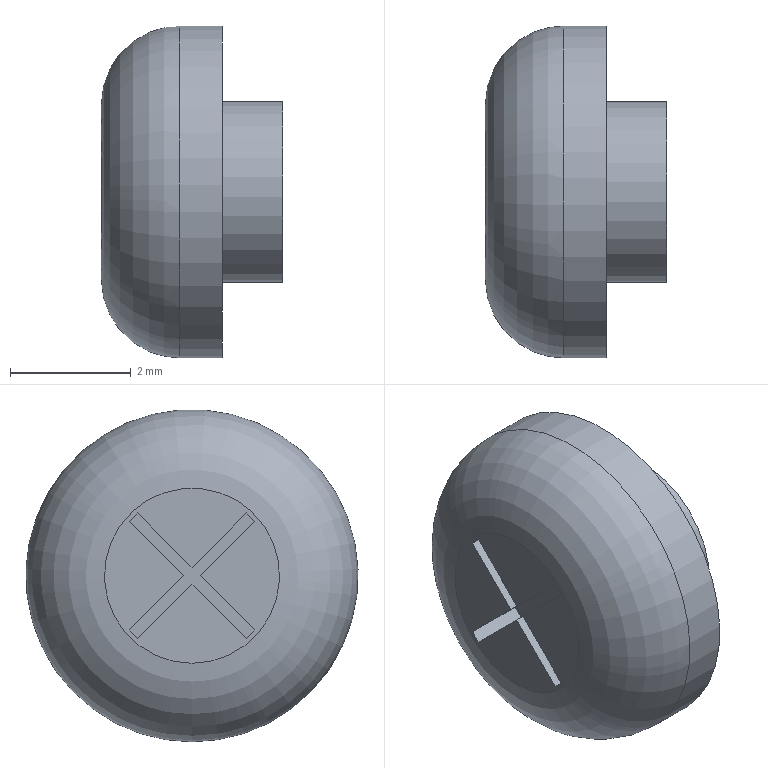Part | STEP file | 1 solid | 19 faces | box 3 x 5.5 x 5.5 mm | volume 47.924 mm3 | plane 16 | cylinder 2 | torus 1 | commonest cylinder face diameters 3 x1 5.5 x1
STEP:
#1=CARTESIAN_POINT('',(0.,0.,0.));
#2=DIRECTION('',(0.,0.,1.));
#3=DIRECTION('',(1.,0.,0.));
#4=AXIS2_PLACEMENT_3D('',#1,#2,#3);
#5=CARTESIAN_POINT('',(0.,0.,-1.5));
#6=VERTEX_POINT('',#5);
#7=CARTESIAN_POINT('',(0.,0.,0.));
#8=DIRECTION('',(-1.,0.,0.));
#9=DIRECTION('',(0.,0.,-1.));
#10=AXIS2_PLACEMENT_3D('',#7,#8,#9);
#11=CIRCLE('',#10,1.5);
#12=CARTESIAN_POINT('',(0.,0.,0.));
#13=DIRECTION('',(1.,0.,0.));
#14=DIRECTION('',(0.,0.,-1.));
#15=AXIS2_PLACEMENT_3D('',#12,#13,#14);
#16=PLANE('',#15);
#17=CARTESIAN_POINT('',(1.5,0.));
#18=CARTESIAN_POINT('',(1.5,-2.598));
#19=CARTESIAN_POINT('',(-0.75,-1.299));
#20=CARTESIAN_POINT('',(-3.,0.));
#21=CARTESIAN_POINT('',(-0.75,1.299));
#22=CARTESIAN_POINT('',(1.5,2.598));
#23=CARTESIAN_POINT('',(1.5,0.));
#24=(BOUNDED_CURVE()B_SPLINE_CURVE(2,(#17,#18,#19,#20,#21,#22,#23),.UNSPECIFIED.,.T.,.F.)B_SPLINE_CURVE_WITH_KNOTS((1,2,2,2,2,1),(-2.094,0.,2.094,4.189,6.283,8.378),.UNSPECIFIED.)CURVE()GEOMETRIC_REPRESENTATION_ITEM()RATIONAL_B_SPLINE_CURVE((1.,0.5,1.,0.5,1.,0.5,1.))REPRESENTATION_ITEM(''));
#25=(GEOMETRIC_REPRESENTATION_CONTEXT(2)PARAMETRIC_REPRESENTATION_CONTEXT()REPRESENTATION_CONTEXT('',''));
#26=DEFINITIONAL_REPRESENTATION('',(#24),#25);
#27=PCURVE('',#16,#26);
#28=CARTESIAN_POINT('',(-2.15,0.,0.));
#29=DIRECTION('',(1.,0.,0.));
#30=DIRECTION('',(0.,0.,-1.));
#31=AXIS2_PLACEMENT_3D('',#28,#29,#30);
#32=CYLINDRICAL_SURFACE('',#31,1.5);
#33=CARTESIAN_POINT('',(6.283,2.15));
#34=DIRECTION('',(-1.,0.));
#35=VECTOR('',#34,1.);
#36=LINE('',#33,#35);
#37=(GEOMETRIC_REPRESENTATION_CONTEXT(2)PARAMETRIC_REPRESENTATION_CONTEXT()REPRESENTATION_CONTEXT('',''));
#38=DEFINITIONAL_REPRESENTATION('',(#36),#37);
#39=PCURVE('',#32,#38);
#40=SURFACE_CURVE('',#11,(#27,#39),.PCURVE_S1.);
#41=EDGE_CURVE('',#6,#6,#40,.T.);
#42=ORIENTED_EDGE('',*,*,#41,.T.);
#43=EDGE_LOOP('',(#42));
#44=FACE_BOUND('',#43,.T.);
#45=CARTESIAN_POINT('',(0.,0.,-2.75));
#46=VERTEX_POINT('',#45);
#47=CARTESIAN_POINT('',(0.,0.,0.));
#48=DIRECTION('',(1.,0.,0.));
#49=DIRECTION('',(0.,0.,-1.));
#50=AXIS2_PLACEMENT_3D('',#47,#48,#49);
#51=CIRCLE('',#50,2.75);
#52=CARTESIAN_POINT('',(0.,0.));
#53=DIRECTION('',(1.,0.));
#54=AXIS2_PLACEMENT_2D('',#52,#53);
#55=CIRCLE('',#54,2.75);
#56=(GEOMETRIC_REPRESENTATION_CONTEXT(2)PARAMETRIC_REPRESENTATION_CONTEXT()REPRESENTATION_CONTEXT('',''));
#57=DEFINITIONAL_REPRESENTATION('',(#55),#56);
#58=PCURVE('',#16,#57);
#59=CARTESIAN_POINT('',(-2.15,0.,0.));
#60=DIRECTION('',(1.,0.,0.));
#61=DIRECTION('',(0.,0.,-1.));
#62=AXIS2_PLACEMENT_3D('',#59,#60,#61);
#63=CYLINDRICAL_SURFACE('',#62,2.75);
#64=CARTESIAN_POINT('',(0.,2.15));
#65=DIRECTION('',(1.,0.));
#66=VECTOR('',#65,1.);
#67=LINE('',#64,#66);
#68=(GEOMETRIC_REPRESENTATION_CONTEXT(2)PARAMETRIC_REPRESENTATION_CONTEXT()REPRESENTATION_CONTEXT('',''));
#69=DEFINITIONAL_REPRESENTATION('',(#67),#68);
#70=PCURVE('',#63,#69);
#71=SURFACE_CURVE('',#51,(#58,#70),.PCURVE_S1.);
#72=EDGE_CURVE('',#46,#46,#71,.T.);
#73=ORIENTED_EDGE('',*,*,#72,.T.);
#74=EDGE_LOOP('',(#73));
#75=FACE_BOUND('',#74,.T.);
#76=ADVANCED_FACE('',(#44,#75),#16,.T.);
#77=CARTESIAN_POINT('',(1.,0.,-1.5));
#78=VERTEX_POINT('',#77);
#79=CARTESIAN_POINT('',(1.,0.,0.));
#80=DIRECTION('',(-1.,0.,0.));
#81=DIRECTION('',(0.,0.,-1.));
#82=AXIS2_PLACEMENT_3D('',#79,#80,#81);
#83=CIRCLE('',#82,1.5);
#84=CARTESIAN_POINT('',(6.283,3.15));
#85=DIRECTION('',(-1.,0.));
#86=VECTOR('',#85,1.);
#87=LINE('',#84,#86);
#88=(GEOMETRIC_REPRESENTATION_CONTEXT(2)PARAMETRIC_REPRESENTATION_CONTEXT()REPRESENTATION_CONTEXT('',''));
#89=DEFINITIONAL_REPRESENTATION('',(#87),#88);
#90=PCURVE('',#32,#89);
#91=CARTESIAN_POINT('',(1.,0.,0.));
#92=DIRECTION('',(1.,0.,0.));
#93=DIRECTION('',(0.,0.,-1.));
#94=AXIS2_PLACEMENT_3D('',#91,#92,#93);
#95=PLANE('',#94);
#96=CARTESIAN_POINT('',(1.5,0.));
#97=CARTESIAN_POINT('',(1.5,-2.598));
#98=CARTESIAN_POINT('',(-0.75,-1.299));
#99=CARTESIAN_POINT('',(-3.,0.));
#100=CARTESIAN_POINT('',(-0.75,1.299));
#101=CARTESIAN_POINT('',(1.5,2.598));
#102=CARTESIAN_POINT('',(1.5,0.));
#103=(BOUNDED_CURVE()B_SPLINE_CURVE(2,(#96,#97,#98,#99,#100,#101,#102),.UNSPECIFIED.,.T.,.F.)B_SPLINE_CURVE_WITH_KNOTS((1,2,2,2,2,1),(-2.094,0.,2.094,4.189,6.283,8.378),.UNSPECIFIED.)CURVE()GEOMETRIC_REPRESENTATION_ITEM()RATIONAL_B_SPLINE_CURVE((1.,0.5,1.,0.5,1.,0.5,1.))REPRESENTATION_ITEM(''));
#104=(GEOMETRIC_REPRESENTATION_CONTEXT(2)PARAMETRIC_REPRESENTATION_CONTEXT()REPRESENTATION_CONTEXT('',''));
#105=DEFINITIONAL_REPRESENTATION('',(#103),#104);
#106=PCURVE('',#95,#105);
#107=SURFACE_CURVE('',#83,(#90,#106),.PCURVE_S1.);
#108=EDGE_CURVE('',#78,#78,#107,.T.);
#109=ORIENTED_EDGE('',*,*,#108,.T.);
#110=CARTESIAN_POINT('',(0.,0.,-1.5));
#111=CARTESIAN_POINT('',(1.,0.,-1.5));
#112=B_SPLINE_CURVE_WITH_KNOTS('',1,(#110,#111),.UNSPECIFIED.,.F.,.F.,(2,2),(2.15,3.15),.PIECEWISE_BEZIER_KNOTS.);
#113=CARTESIAN_POINT('',(0.,0.));
#114=DIRECTION('',(0.,1.));
#115=VECTOR('',#114,1.);
#116=LINE('',#113,#115);
#117=(GEOMETRIC_REPRESENTATION_CONTEXT(2)PARAMETRIC_REPRESENTATION_CONTEXT()REPRESENTATION_CONTEXT('',''));
#118=DEFINITIONAL_REPRESENTATION('',(#116),#117);
#119=PCURVE('',#32,#118);
#120=CARTESIAN_POINT('',(6.283,0.));
#121=DIRECTION('',(0.,1.));
#122=VECTOR('',#121,1.);
#123=LINE('',#120,#122);
#124=(GEOMETRIC_REPRESENTATION_CONTEXT(2)PARAMETRIC_REPRESENTATION_CONTEXT()REPRESENTATION_CONTEXT('',''));
#125=DEFINITIONAL_REPRESENTATION('',(#123),#124);
#126=PCURVE('',#32,#125);
#127=SEAM_CURVE('',#112,(#119,#126),.PCURVE_S1.);
#128=EDGE_CURVE('',#6,#78,#127,.T.);
#129=ORIENTED_EDGE('',*,*,#128,.F.);
#130=ORIENTED_EDGE('',*,*,#41,.F.);
#131=ORIENTED_EDGE('',*,*,#128,.T.);
#132=EDGE_LOOP('',(#109,#129,#130,#131));
#133=FACE_BOUND('',#132,.T.);
#134=ADVANCED_FACE('',(#133),#32,.T.);
#135=CARTESIAN_POINT('',(-0.7,0.,-2.75));
#136=VERTEX_POINT('',#135);
#137=CARTESIAN_POINT('',(-0.7,0.,0.));
#138=DIRECTION('',(1.,0.,0.));
#139=DIRECTION('',(0.,0.,-1.));
#140=AXIS2_PLACEMENT_3D('',#137,#138,#139);
#141=CIRCLE('',#140,2.75);
#142=CARTESIAN_POINT('',(0.,1.45));
#143=DIRECTION('',(1.,0.));
#144=VECTOR('',#143,1.);
#145=LINE('',#142,#144);
#146=(GEOMETRIC_REPRESENTATION_CONTEXT(2)PARAMETRIC_REPRESENTATION_CONTEXT()REPRESENTATION_CONTEXT('',''));
#147=DEFINITIONAL_REPRESENTATION('',(#145),#146);
#148=PCURVE('',#63,#147);
#149=CARTESIAN_POINT('',(-0.7,0.,0.));
#150=DIRECTION('',(1.,0.,0.));
#151=DIRECTION('',(0.,0.,-1.));
#152=AXIS2_PLACEMENT_3D('',#149,#150,#151);
#153=TOROIDAL_SURFACE('',#152,1.45,1.3);
#154=CARTESIAN_POINT('',(0.,6.283));
#155=DIRECTION('',(1.,0.));
#156=VECTOR('',#155,1.);
#157=LINE('',#154,#156);
#158=(GEOMETRIC_REPRESENTATION_CONTEXT(2)PARAMETRIC_REPRESENTATION_CONTEXT()REPRESENTATION_CONTEXT('',''));
#159=DEFINITIONAL_REPRESENTATION('',(#157),#158);
#160=PCURVE('',#153,#159);
#161=SURFACE_CURVE('',#141,(#148,#160),.PCURVE_S1.);
#162=EDGE_CURVE('',#136,#136,#161,.T.);
#163=ORIENTED_EDGE('',*,*,#162,.T.);
#164=CARTESIAN_POINT('',(-0.7,0.,-2.75));
#165=CARTESIAN_POINT('',(0.,0.,-2.75));
#166=B_SPLINE_CURVE_WITH_KNOTS('',1,(#164,#165),.UNSPECIFIED.,.F.,.F.,(2,2),(1.45,2.15),.PIECEWISE_BEZIER_KNOTS.);
#167=CARTESIAN_POINT('',(6.283,0.));
#168=DIRECTION('',(0.,1.));
#169=VECTOR('',#168,1.);
#170=LINE('',#167,#169);
#171=(GEOMETRIC_REPRESENTATION_CONTEXT(2)PARAMETRIC_REPRESENTATION_CONTEXT()REPRESENTATION_CONTEXT('',''));
#172=DEFINITIONAL_REPRESENTATION('',(#170),#171);
#173=PCURVE('',#63,#172);
#174=CARTESIAN_POINT('',(0.,0.));
#175=DIRECTION('',(0.,1.));
#176=VECTOR('',#175,1.);
#177=LINE('',#174,#176);
#178=(GEOMETRIC_REPRESENTATION_CONTEXT(2)PARAMETRIC_REPRESENTATION_CONTEXT()REPRESENTATION_CONTEXT('',''));
#179=DEFINITIONAL_REPRESENTATION('',(#177),#178);
#180=PCURVE('',#63,#179);
#181=SEAM_CURVE('',#166,(#173,#180),.PCURVE_S1.);
#182=EDGE_CURVE('',#136,#46,#181,.T.);
#183=ORIENTED_EDGE('',*,*,#182,.T.);
#184=ORIENTED_EDGE('',*,*,#72,.F.);
#185=ORIENTED_EDGE('',*,*,#182,.F.);
#186=EDGE_LOOP('',(#163,#183,#184,#185));
#187=FACE_BOUND('',#186,.T.);
#188=ADVANCED_FACE('',(#187),#63,.T.);
#189=ORIENTED_EDGE('',*,*,#108,.F.);
#190=EDGE_LOOP('',(#189));
#191=FACE_BOUND('',#190,.T.);
#192=ADVANCED_FACE('',(#191),#95,.T.);
#193=ORIENTED_EDGE('',*,*,#162,.F.);
#194=CARTESIAN_POINT('',(-2.,0.,-1.45));
#195=VERTEX_POINT('',#194);
#196=CARTESIAN_POINT('',(-2.,0.,-1.45));
#197=CARTESIAN_POINT('',(-2.,0.,-1.798));
#198=CARTESIAN_POINT('',(-1.889,0.,-2.136));
#199=CARTESIAN_POINT('',(-1.677,0.,-2.427));
#200=CARTESIAN_POINT('',(-1.386,0.,-2.639));
#201=CARTESIAN_POINT('',(-1.048,0.,-2.75));
#202=CARTESIAN_POINT('',(-0.7,0.,-2.75));
#203=(BOUNDED_CURVE()B_SPLINE_CURVE(6,(#196,#197,#198,#199,#200,#201,#202),.UNSPECIFIED.,.F.,.F.)B_SPLINE_CURVE_WITH_KNOTS((7,7),(-1.571,0.),.PIECEWISE_BEZIER_KNOTS.)CURVE()GEOMETRIC_REPRESENTATION_ITEM()RATIONAL_B_SPLINE_CURVE((1.031,1.01,0.9979,0.994,0.9979,1.01,1.031))REPRESENTATION_ITEM(''));
#204=CARTESIAN_POINT('',(0.,6.283));
#205=DIRECTION('',(0.,1.));
#206=VECTOR('',#205,1.);
#207=LINE('',#204,#206);
#208=(GEOMETRIC_REPRESENTATION_CONTEXT(2)PARAMETRIC_REPRESENTATION_CONTEXT()REPRESENTATION_CONTEXT('',''));
#209=DEFINITIONAL_REPRESENTATION('',(#207),#208);
#210=PCURVE('',#153,#209);
#211=CARTESIAN_POINT('',(6.283,6.283));
#212=DIRECTION('',(0.,1.));
#213=VECTOR('',#212,1.);
#214=LINE('',#211,#213);
#215=(GEOMETRIC_REPRESENTATION_CONTEXT(2)PARAMETRIC_REPRESENTATION_CONTEXT()REPRESENTATION_CONTEXT('',''));
#216=DEFINITIONAL_REPRESENTATION('',(#214),#215);
#217=PCURVE('',#153,#216);
#218=SEAM_CURVE('',#203,(#210,#217),.PCURVE_S1.);
#219=EDGE_CURVE('',#195,#136,#218,.T.);
#220=ORIENTED_EDGE('',*,*,#219,.F.);
#221=CARTESIAN_POINT('',(-2.,0.,0.));
#222=DIRECTION('',(1.,0.,0.));
#223=DIRECTION('',(0.,0.,-1.));
#224=AXIS2_PLACEMENT_3D('',#221,#222,#223);
#225=CIRCLE('',#224,1.45);
#226=CARTESIAN_POINT('',(0.,4.712));
#227=DIRECTION('',(1.,0.));
#228=VECTOR('',#227,1.);
#229=LINE('',#226,#228);
#230=(GEOMETRIC_REPRESENTATION_CONTEXT(2)PARAMETRIC_REPRESENTATION_CONTEXT()REPRESENTATION_CONTEXT('',''));
#231=DEFINITIONAL_REPRESENTATION('',(#229),#230);
#232=PCURVE('',#153,#231);
#233=CARTESIAN_POINT('',(-2.,0.,0.));
#234=DIRECTION('',(1.,0.,0.));
#235=DIRECTION('',(0.,0.,-1.));
#236=AXIS2_PLACEMENT_3D('',#233,#234,#235);
#237=PLANE('',#236);
#238=CARTESIAN_POINT('',(0.,0.));
#239=DIRECTION('',(1.,0.));
#240=AXIS2_PLACEMENT_2D('',#238,#239);
#241=CIRCLE('',#240,1.45);
#242=(GEOMETRIC_REPRESENTATION_CONTEXT(2)PARAMETRIC_REPRESENTATION_CONTEXT()REPRESENTATION_CONTEXT('',''));
#243=DEFINITIONAL_REPRESENTATION('',(#241),#242);
#244=PCURVE('',#237,#243);
#245=SURFACE_CURVE('',#225,(#232,#244),.PCURVE_S1.);
#246=EDGE_CURVE('',#195,#195,#245,.T.);
#247=ORIENTED_EDGE('',*,*,#246,.T.);
#248=ORIENTED_EDGE('',*,*,#219,.T.);
#249=EDGE_LOOP('',(#193,#220,#247,#248));
#250=FACE_BOUND('',#249,.T.);
#251=ADVANCED_FACE('',(#250),#153,.T.);
#252=CARTESIAN_POINT('',(-2.,1.039,0.898));
#253=VERTEX_POINT('',#252);
#254=CARTESIAN_POINT('',(-2.,0.1414,0.));
#255=VERTEX_POINT('',#254);
#256=CARTESIAN_POINT('',(-2.,1.039,0.898));
#257=DIRECTION('',(0.,-0.7071,-0.7071));
#258=VECTOR('',#257,1.);
#259=LINE('',#256,#258);
#260=CARTESIAN_POINT('',(-0.898,1.039));
#261=DIRECTION('',(0.7071,-0.7071));
#262=VECTOR('',#261,1.);
#263=LINE('',#260,#262);
#264=(GEOMETRIC_REPRESENTATION_CONTEXT(2)PARAMETRIC_REPRESENTATION_CONTEXT()REPRESENTATION_CONTEXT('',''));
#265=DEFINITIONAL_REPRESENTATION('',(#263),#264);
#266=PCURVE('',#237,#265);
#267=CARTESIAN_POINT('',(-2.,1.039,0.898));
#268=DIRECTION('',(0.,0.7071,-0.7071));
#269=DIRECTION('',(0.,0.7071,0.7071));
#270=AXIS2_PLACEMENT_3D('',#267,#268,#269);
#271=PLANE('',#270);
#272=CARTESIAN_POINT('',(0.,0.));
#273=DIRECTION('',(-1.,0.));
#274=VECTOR('',#273,1.);
#275=LINE('',#272,#274);
#276=(GEOMETRIC_REPRESENTATION_CONTEXT(2)PARAMETRIC_REPRESENTATION_CONTEXT()REPRESENTATION_CONTEXT('',''));
#277=DEFINITIONAL_REPRESENTATION('',(#275),#276);
#278=PCURVE('',#271,#277);
#279=SURFACE_CURVE('',#259,(#266,#278),.PCURVE_S1.);
#280=EDGE_CURVE('',#253,#255,#279,.T.);
#281=ORIENTED_EDGE('',*,*,#280,.F.);
#282=CARTESIAN_POINT('',(-2.,0.898,1.039));
#283=VERTEX_POINT('',#282);
#284=CARTESIAN_POINT('',(-2.,0.898,1.039));
#285=DIRECTION('',(0.,0.7071,-0.7071));
#286=VECTOR('',#285,1.);
#287=LINE('',#284,#286);
#288=CARTESIAN_POINT('',(-1.039,0.898));
#289=DIRECTION('',(0.7071,0.7071));
#290=VECTOR('',#289,1.);
#291=LINE('',#288,#290);
#292=(GEOMETRIC_REPRESENTATION_CONTEXT(2)PARAMETRIC_REPRESENTATION_CONTEXT()REPRESENTATION_CONTEXT('',''));
#293=DEFINITIONAL_REPRESENTATION('',(#291),#292);
#294=PCURVE('',#237,#293);
#295=CARTESIAN_POINT('',(-2.,0.898,1.039));
#296=DIRECTION('',(0.,0.7071,0.7071));
#297=DIRECTION('',(0.,-0.7071,0.7071));
#298=AXIS2_PLACEMENT_3D('',#295,#296,#297);
#299=PLANE('',#298);
#300=CARTESIAN_POINT('',(0.,0.));
#301=DIRECTION('',(-1.,0.));
#302=VECTOR('',#301,1.);
#303=LINE('',#300,#302);
#304=(GEOMETRIC_REPRESENTATION_CONTEXT(2)PARAMETRIC_REPRESENTATION_CONTEXT()REPRESENTATION_CONTEXT('',''));
#305=DEFINITIONAL_REPRESENTATION('',(#303),#304);
#306=PCURVE('',#299,#305);
#307=SURFACE_CURVE('',#287,(#294,#306),.PCURVE_S1.);
#308=EDGE_CURVE('',#283,#253,#307,.T.);
#309=ORIENTED_EDGE('',*,*,#308,.F.);
#310=CARTESIAN_POINT('',(-2.,0.,0.1414));
#311=VERTEX_POINT('',#310);
#312=CARTESIAN_POINT('',(-2.,0.,0.1414));
#313=DIRECTION('',(0.,0.7071,0.7071));
#314=VECTOR('',#313,1.);
#315=LINE('',#312,#314);
#316=CARTESIAN_POINT('',(-0.1414,0.));
#317=DIRECTION('',(-0.7071,0.7071));
#318=VECTOR('',#317,1.);
#319=LINE('',#316,#318);
#320=(GEOMETRIC_REPRESENTATION_CONTEXT(2)PARAMETRIC_REPRESENTATION_CONTEXT()REPRESENTATION_CONTEXT('',''));
#321=DEFINITIONAL_REPRESENTATION('',(#319),#320);
#322=PCURVE('',#237,#321);
#323=CARTESIAN_POINT('',(-2.,0.,0.1414));
#324=DIRECTION('',(0.,-0.7071,0.7071));
#325=DIRECTION('',(0.,-0.7071,-0.7071));
#326=AXIS2_PLACEMENT_3D('',#323,#324,#325);
#327=PLANE('',#326);
#328=CARTESIAN_POINT('',(0.,0.));
#329=DIRECTION('',(-1.,0.));
#330=VECTOR('',#329,1.);
#331=LINE('',#328,#330);
#332=(GEOMETRIC_REPRESENTATION_CONTEXT(2)PARAMETRIC_REPRESENTATION_CONTEXT()REPRESENTATION_CONTEXT('',''));
#333=DEFINITIONAL_REPRESENTATION('',(#331),#332);
#334=PCURVE('',#327,#333);
#335=SURFACE_CURVE('',#315,(#322,#334),.PCURVE_S1.);
#336=EDGE_CURVE('',#311,#283,#335,.T.);
#337=ORIENTED_EDGE('',*,*,#336,.F.);
#338=CARTESIAN_POINT('',(-2.,-0.898,1.039));
#339=VERTEX_POINT('',#338);
#340=CARTESIAN_POINT('',(-2.,-0.898,1.039));
#341=DIRECTION('',(0.,0.7071,-0.7071));
#342=VECTOR('',#341,1.);
#343=LINE('',#340,#342);
#344=CARTESIAN_POINT('',(-1.039,-0.898));
#345=DIRECTION('',(0.7071,0.7071));
#346=VECTOR('',#345,1.);
#347=LINE('',#344,#346);
#348=(GEOMETRIC_REPRESENTATION_CONTEXT(2)PARAMETRIC_REPRESENTATION_CONTEXT()REPRESENTATION_CONTEXT('',''));
#349=DEFINITIONAL_REPRESENTATION('',(#347),#348);
#350=PCURVE('',#237,#349);
#351=CARTESIAN_POINT('',(-2.,-0.898,1.039));
#352=DIRECTION('',(0.,0.7071,0.7071));
#353=DIRECTION('',(0.,-0.7071,0.7071));
#354=AXIS2_PLACEMENT_3D('',#351,#352,#353);
#355=PLANE('',#354);
#356=CARTESIAN_POINT('',(0.,0.));
#357=DIRECTION('',(-1.,0.));
#358=VECTOR('',#357,1.);
#359=LINE('',#356,#358);
#360=(GEOMETRIC_REPRESENTATION_CONTEXT(2)PARAMETRIC_REPRESENTATION_CONTEXT()REPRESENTATION_CONTEXT('',''));
#361=DEFINITIONAL_REPRESENTATION('',(#359),#360);
#362=PCURVE('',#355,#361);
#363=SURFACE_CURVE('',#343,(#350,#362),.PCURVE_S1.);
#364=EDGE_CURVE('',#339,#311,#363,.T.);
#365=ORIENTED_EDGE('',*,*,#364,.F.);
#366=CARTESIAN_POINT('',(-2.,-1.039,0.898));
#367=VERTEX_POINT('',#366);
#368=CARTESIAN_POINT('',(-2.,-1.039,0.898));
#369=DIRECTION('',(0.,0.7071,0.7071));
#370=VECTOR('',#369,1.);
#371=LINE('',#368,#370);
#372=CARTESIAN_POINT('',(-0.898,-1.039));
#373=DIRECTION('',(-0.7071,0.7071));
#374=VECTOR('',#373,1.);
#375=LINE('',#372,#374);
#376=(GEOMETRIC_REPRESENTATION_CONTEXT(2)PARAMETRIC_REPRESENTATION_CONTEXT()REPRESENTATION_CONTEXT('',''));
#377=DEFINITIONAL_REPRESENTATION('',(#375),#376);
#378=PCURVE('',#237,#377);
#379=CARTESIAN_POINT('',(-2.,-1.039,0.898));
#380=DIRECTION('',(0.,-0.7071,0.7071));
#381=DIRECTION('',(0.,-0.7071,-0.7071));
#382=AXIS2_PLACEMENT_3D('',#379,#380,#381);
#383=PLANE('',#382);
#384=CARTESIAN_POINT('',(0.,0.));
#385=DIRECTION('',(-1.,0.));
#386=VECTOR('',#385,1.);
#387=LINE('',#384,#386);
#388=(GEOMETRIC_REPRESENTATION_CONTEXT(2)PARAMETRIC_REPRESENTATION_CONTEXT()REPRESENTATION_CONTEXT('',''));
#389=DEFINITIONAL_REPRESENTATION('',(#387),#388);
#390=PCURVE('',#383,#389);
#391=SURFACE_CURVE('',#371,(#378,#390),.PCURVE_S1.);
#392=EDGE_CURVE('',#367,#339,#391,.T.);
#393=ORIENTED_EDGE('',*,*,#392,.F.);
#394=CARTESIAN_POINT('',(-2.,-0.1414,0.));
#395=VERTEX_POINT('',#394);
#396=CARTESIAN_POINT('',(-2.,-0.1414,0.));
#397=DIRECTION('',(0.,-0.7071,0.7071));
#398=VECTOR('',#397,1.);
#399=LINE('',#396,#398);
#400=CARTESIAN_POINT('',(0.,-0.1414));
#401=DIRECTION('',(-0.7071,-0.7071));
#402=VECTOR('',#401,1.);
#403=LINE('',#400,#402);
#404=(GEOMETRIC_REPRESENTATION_CONTEXT(2)PARAMETRIC_REPRESENTATION_CONTEXT()REPRESENTATION_CONTEXT('',''));
#405=DEFINITIONAL_REPRESENTATION('',(#403),#404);
#406=PCURVE('',#237,#405);
#407=CARTESIAN_POINT('',(-2.,-0.1414,0.));
#408=DIRECTION('',(0.,-0.7071,-0.7071));
#409=DIRECTION('',(0.,0.7071,-0.7071));
#410=AXIS2_PLACEMENT_3D('',#407,#408,#409);
#411=PLANE('',#410);
#412=CARTESIAN_POINT('',(0.,0.));
#413=DIRECTION('',(-1.,0.));
#414=VECTOR('',#413,1.);
#415=LINE('',#412,#414);
#416=(GEOMETRIC_REPRESENTATION_CONTEXT(2)PARAMETRIC_REPRESENTATION_CONTEXT()REPRESENTATION_CONTEXT('',''));
#417=DEFINITIONAL_REPRESENTATION('',(#415),#416);
#418=PCURVE('',#411,#417);
#419=SURFACE_CURVE('',#399,(#406,#418),.PCURVE_S1.);
#420=EDGE_CURVE('',#395,#367,#419,.T.);
#421=ORIENTED_EDGE('',*,*,#420,.F.);
#422=CARTESIAN_POINT('',(-2.,-1.039,-0.898));
#423=VERTEX_POINT('',#422);
#424=CARTESIAN_POINT('',(-2.,-1.039,-0.898));
#425=DIRECTION('',(0.,0.7071,0.7071));
#426=VECTOR('',#425,1.);
#427=LINE('',#424,#426);
#428=CARTESIAN_POINT('',(0.898,-1.039));
#429=DIRECTION('',(-0.7071,0.7071));
#430=VECTOR('',#429,1.);
#431=LINE('',#428,#430);
#432=(GEOMETRIC_REPRESENTATION_CONTEXT(2)PARAMETRIC_REPRESENTATION_CONTEXT()REPRESENTATION_CONTEXT('',''));
#433=DEFINITIONAL_REPRESENTATION('',(#431),#432);
#434=PCURVE('',#237,#433);
#435=CARTESIAN_POINT('',(-2.,-1.039,-0.898));
#436=DIRECTION('',(0.,-0.7071,0.7071));
#437=DIRECTION('',(0.,-0.7071,-0.7071));
#438=AXIS2_PLACEMENT_3D('',#435,#436,#437);
#439=PLANE('',#438);
#440=CARTESIAN_POINT('',(0.,0.));
#441=DIRECTION('',(-1.,0.));
#442=VECTOR('',#441,1.);
#443=LINE('',#440,#442);
#444=(GEOMETRIC_REPRESENTATION_CONTEXT(2)PARAMETRIC_REPRESENTATION_CONTEXT()REPRESENTATION_CONTEXT('',''));
#445=DEFINITIONAL_REPRESENTATION('',(#443),#444);
#446=PCURVE('',#439,#445);
#447=SURFACE_CURVE('',#427,(#434,#446),.PCURVE_S1.);
#448=EDGE_CURVE('',#423,#395,#447,.T.);
#449=ORIENTED_EDGE('',*,*,#448,.F.);
#450=CARTESIAN_POINT('',(-2.,-0.898,-1.039));
#451=VERTEX_POINT('',#450);
#452=CARTESIAN_POINT('',(-2.,-0.898,-1.039));
#453=DIRECTION('',(0.,-0.7071,0.7071));
#454=VECTOR('',#453,1.);
#455=LINE('',#452,#454);
#456=CARTESIAN_POINT('',(1.039,-0.898));
#457=DIRECTION('',(-0.7071,-0.7071));
#458=VECTOR('',#457,1.);
#459=LINE('',#456,#458);
#460=(GEOMETRIC_REPRESENTATION_CONTEXT(2)PARAMETRIC_REPRESENTATION_CONTEXT()REPRESENTATION_CONTEXT('',''));
#461=DEFINITIONAL_REPRESENTATION('',(#459),#460);
#462=PCURVE('',#237,#461);
#463=CARTESIAN_POINT('',(-2.,-0.898,-1.039));
#464=DIRECTION('',(0.,-0.7071,-0.7071));
#465=DIRECTION('',(0.,0.7071,-0.7071));
#466=AXIS2_PLACEMENT_3D('',#463,#464,#465);
#467=PLANE('',#466);
#468=CARTESIAN_POINT('',(0.,0.));
#469=DIRECTION('',(-1.,0.));
#470=VECTOR('',#469,1.);
#471=LINE('',#468,#470);
#472=(GEOMETRIC_REPRESENTATION_CONTEXT(2)PARAMETRIC_REPRESENTATION_CONTEXT()REPRESENTATION_CONTEXT('',''));
#473=DEFINITIONAL_REPRESENTATION('',(#471),#472);
#474=PCURVE('',#467,#473);
#475=SURFACE_CURVE('',#455,(#462,#474),.PCURVE_S1.);
#476=EDGE_CURVE('',#451,#423,#475,.T.);
#477=ORIENTED_EDGE('',*,*,#476,.F.);
#478=CARTESIAN_POINT('',(-2.,0.,-0.1414));
#479=VERTEX_POINT('',#478);
#480=CARTESIAN_POINT('',(-2.,0.,-0.1414));
#481=DIRECTION('',(0.,-0.7071,-0.7071));
#482=VECTOR('',#481,1.);
#483=LINE('',#480,#482);
#484=CARTESIAN_POINT('',(0.1414,0.));
#485=DIRECTION('',(0.7071,-0.7071));
#486=VECTOR('',#485,1.);
#487=LINE('',#484,#486);
#488=(GEOMETRIC_REPRESENTATION_CONTEXT(2)PARAMETRIC_REPRESENTATION_CONTEXT()REPRESENTATION_CONTEXT('',''));
#489=DEFINITIONAL_REPRESENTATION('',(#487),#488);
#490=PCURVE('',#237,#489);
#491=CARTESIAN_POINT('',(-2.,0.,-0.1414));
#492=DIRECTION('',(0.,0.7071,-0.7071));
#493=DIRECTION('',(0.,0.7071,0.7071));
#494=AXIS2_PLACEMENT_3D('',#491,#492,#493);
#495=PLANE('',#494);
#496=CARTESIAN_POINT('',(0.,0.));
#497=DIRECTION('',(-1.,0.));
#498=VECTOR('',#497,1.);
#499=LINE('',#496,#498);
#500=(GEOMETRIC_REPRESENTATION_CONTEXT(2)PARAMETRIC_REPRESENTATION_CONTEXT()REPRESENTATION_CONTEXT('',''));
#501=DEFINITIONAL_REPRESENTATION('',(#499),#500);
#502=PCURVE('',#495,#501);
#503=SURFACE_CURVE('',#483,(#490,#502),.PCURVE_S1.);
#504=EDGE_CURVE('',#479,#451,#503,.T.);
#505=ORIENTED_EDGE('',*,*,#504,.F.);
#506=CARTESIAN_POINT('',(-2.,0.898,-1.039));
#507=VERTEX_POINT('',#506);
#508=CARTESIAN_POINT('',(-2.,0.898,-1.039));
#509=DIRECTION('',(0.,-0.7071,0.7071));
#510=VECTOR('',#509,1.);
#511=LINE('',#508,#510);
#512=CARTESIAN_POINT('',(1.039,0.898));
#513=DIRECTION('',(-0.7071,-0.7071));
#514=VECTOR('',#513,1.);
#515=LINE('',#512,#514);
#516=(GEOMETRIC_REPRESENTATION_CONTEXT(2)PARAMETRIC_REPRESENTATION_CONTEXT()REPRESENTATION_CONTEXT('',''));
#517=DEFINITIONAL_REPRESENTATION('',(#515),#516);
#518=PCURVE('',#237,#517);
#519=CARTESIAN_POINT('',(-2.,0.898,-1.039));
#520=DIRECTION('',(0.,-0.7071,-0.7071));
#521=DIRECTION('',(0.,0.7071,-0.7071));
#522=AXIS2_PLACEMENT_3D('',#519,#520,#521);
#523=PLANE('',#522);
#524=CARTESIAN_POINT('',(0.,0.));
#525=DIRECTION('',(-1.,0.));
#526=VECTOR('',#525,1.);
#527=LINE('',#524,#526);
#528=(GEOMETRIC_REPRESENTATION_CONTEXT(2)PARAMETRIC_REPRESENTATION_CONTEXT()REPRESENTATION_CONTEXT('',''));
#529=DEFINITIONAL_REPRESENTATION('',(#527),#528);
#530=PCURVE('',#523,#529);
#531=SURFACE_CURVE('',#511,(#518,#530),.PCURVE_S1.);
#532=EDGE_CURVE('',#507,#479,#531,.T.);
#533=ORIENTED_EDGE('',*,*,#532,.F.);
#534=CARTESIAN_POINT('',(-2.,1.039,-0.898));
#535=VERTEX_POINT('',#534);
#536=CARTESIAN_POINT('',(-2.,1.039,-0.898));
#537=DIRECTION('',(0.,-0.7071,-0.7071));
#538=VECTOR('',#537,1.);
#539=LINE('',#536,#538);
#540=CARTESIAN_POINT('',(0.898,1.039));
#541=DIRECTION('',(0.7071,-0.7071));
#542=VECTOR('',#541,1.);
#543=LINE('',#540,#542);
#544=(GEOMETRIC_REPRESENTATION_CONTEXT(2)PARAMETRIC_REPRESENTATION_CONTEXT()REPRESENTATION_CONTEXT('',''));
#545=DEFINITIONAL_REPRESENTATION('',(#543),#544);
#546=PCURVE('',#237,#545);
#547=CARTESIAN_POINT('',(-2.,1.039,-0.898));
#548=DIRECTION('',(0.,0.7071,-0.7071));
#549=DIRECTION('',(0.,0.7071,0.7071));
#550=AXIS2_PLACEMENT_3D('',#547,#548,#549);
#551=PLANE('',#550);
#552=CARTESIAN_POINT('',(0.,0.));
#553=DIRECTION('',(-1.,0.));
#554=VECTOR('',#553,1.);
#555=LINE('',#552,#554);
#556=(GEOMETRIC_REPRESENTATION_CONTEXT(2)PARAMETRIC_REPRESENTATION_CONTEXT()REPRESENTATION_CONTEXT('',''));
#557=DEFINITIONAL_REPRESENTATION('',(#555),#556);
#558=PCURVE('',#551,#557);
#559=SURFACE_CURVE('',#539,(#546,#558),.PCURVE_S1.);
#560=EDGE_CURVE('',#535,#507,#559,.T.);
#561=ORIENTED_EDGE('',*,*,#560,.F.);
#562=CARTESIAN_POINT('',(-2.,0.1414,0.));
#563=DIRECTION('',(0.,0.7071,-0.7071));
#564=VECTOR('',#563,1.);
#565=LINE('',#562,#564);
#566=CARTESIAN_POINT('',(0.,0.1414));
#567=DIRECTION('',(0.7071,0.7071));
#568=VECTOR('',#567,1.);
#569=LINE('',#566,#568);
#570=(GEOMETRIC_REPRESENTATION_CONTEXT(2)PARAMETRIC_REPRESENTATION_CONTEXT()REPRESENTATION_CONTEXT('',''));
#571=DEFINITIONAL_REPRESENTATION('',(#569),#570);
#572=PCURVE('',#237,#571);
#573=CARTESIAN_POINT('',(-2.,0.1414,0.));
#574=DIRECTION('',(0.,0.7071,0.7071));
#575=DIRECTION('',(0.,-0.7071,0.7071));
#576=AXIS2_PLACEMENT_3D('',#573,#574,#575);
#577=PLANE('',#576);
#578=CARTESIAN_POINT('',(0.,0.));
#579=DIRECTION('',(-1.,0.));
#580=VECTOR('',#579,1.);
#581=LINE('',#578,#580);
#582=(GEOMETRIC_REPRESENTATION_CONTEXT(2)PARAMETRIC_REPRESENTATION_CONTEXT()REPRESENTATION_CONTEXT('',''));
#583=DEFINITIONAL_REPRESENTATION('',(#581),#582);
#584=PCURVE('',#577,#583);
#585=SURFACE_CURVE('',#565,(#572,#584),.PCURVE_S1.);
#586=EDGE_CURVE('',#255,#535,#585,.T.);
#587=ORIENTED_EDGE('',*,*,#586,.F.);
#588=EDGE_LOOP('',(#281,#309,#337,#365,#393,#421,#449,#477,#505,#533,#561,#587));
#589=FACE_BOUND('',#588,.T.);
#590=ORIENTED_EDGE('',*,*,#246,.F.);
#591=EDGE_LOOP('',(#590));
#592=FACE_BOUND('',#591,.T.);
#593=ADVANCED_FACE('',(#589,#592),#237,.F.);
#594=CARTESIAN_POINT('',(-1.,0.1414,0.));
#595=VERTEX_POINT('',#594);
#596=CARTESIAN_POINT('',(-2.,0.1414,0.));
#597=DIRECTION('',(1.,0.,0.));
#598=VECTOR('',#597,1.);
#599=LINE('',#596,#598);
#600=CARTESIAN_POINT('',(0.,0.));
#601=DIRECTION('',(0.,1.));
#602=VECTOR('',#601,1.);
#603=LINE('',#600,#602);
#604=(GEOMETRIC_REPRESENTATION_CONTEXT(2)PARAMETRIC_REPRESENTATION_CONTEXT()REPRESENTATION_CONTEXT('',''));
#605=DEFINITIONAL_REPRESENTATION('',(#603),#604);
#606=PCURVE('',#577,#605);
#607=CARTESIAN_POINT('',(-1.27,0.));
#608=DIRECTION('',(0.,1.));
#609=VECTOR('',#608,1.);
#610=LINE('',#607,#609);
#611=(GEOMETRIC_REPRESENTATION_CONTEXT(2)PARAMETRIC_REPRESENTATION_CONTEXT()REPRESENTATION_CONTEXT('',''));
#612=DEFINITIONAL_REPRESENTATION('',(#610),#611);
#613=PCURVE('',#271,#612);
#614=SURFACE_CURVE('',#599,(#606,#613),.PCURVE_S1.);
#615=EDGE_CURVE('',#255,#595,#614,.T.);
#616=ORIENTED_EDGE('',*,*,#615,.F.);
#617=ORIENTED_EDGE('',*,*,#586,.T.);
#618=CARTESIAN_POINT('',(-1.,1.039,-0.898));
#619=VERTEX_POINT('',#618);
#620=CARTESIAN_POINT('',(-2.,1.039,-0.898));
#621=DIRECTION('',(-1.,0.,0.));
#622=VECTOR('',#621,1.);
#623=LINE('',#620,#622);
#624=CARTESIAN_POINT('',(-1.27,0.));
#625=DIRECTION('',(0.,-1.));
#626=VECTOR('',#625,1.);
#627=LINE('',#624,#626);
#628=(GEOMETRIC_REPRESENTATION_CONTEXT(2)PARAMETRIC_REPRESENTATION_CONTEXT()REPRESENTATION_CONTEXT('',''));
#629=DEFINITIONAL_REPRESENTATION('',(#627),#628);
#630=PCURVE('',#577,#629);
#631=CARTESIAN_POINT('',(0.,0.));
#632=DIRECTION('',(0.,-1.));
#633=VECTOR('',#632,1.);
#634=LINE('',#631,#633);
#635=(GEOMETRIC_REPRESENTATION_CONTEXT(2)PARAMETRIC_REPRESENTATION_CONTEXT()REPRESENTATION_CONTEXT('',''));
#636=DEFINITIONAL_REPRESENTATION('',(#634),#635);
#637=PCURVE('',#551,#636);
#638=SURFACE_CURVE('',#623,(#630,#637),.PCURVE_S1.);
#639=EDGE_CURVE('',#619,#535,#638,.T.);
#640=ORIENTED_EDGE('',*,*,#639,.F.);
#641=CARTESIAN_POINT('',(-1.,0.1414,0.));
#642=DIRECTION('',(0.,0.7071,-0.7071));
#643=VECTOR('',#642,1.);
#644=LINE('',#641,#643);
#645=CARTESIAN_POINT('',(0.,1.));
#646=DIRECTION('',(-1.,0.));
#647=VECTOR('',#646,1.);
#648=LINE('',#645,#647);
#649=(GEOMETRIC_REPRESENTATION_CONTEXT(2)PARAMETRIC_REPRESENTATION_CONTEXT()REPRESENTATION_CONTEXT('',''));
#650=DEFINITIONAL_REPRESENTATION('',(#648),#649);
#651=PCURVE('',#577,#650);
#652=CARTESIAN_POINT('',(-1.,0.,0.));
#653=DIRECTION('',(-1.,0.,0.));
#654=DIRECTION('',(0.,0.,1.));
#655=AXIS2_PLACEMENT_3D('',#652,#653,#654);
#656=PLANE('',#655);
#657=CARTESIAN_POINT('',(0.,0.1414));
#658=DIRECTION('',(-0.7071,0.7071));
#659=VECTOR('',#658,1.);
#660=LINE('',#657,#659);
#661=(GEOMETRIC_REPRESENTATION_CONTEXT(2)PARAMETRIC_REPRESENTATION_CONTEXT()REPRESENTATION_CONTEXT('',''));
#662=DEFINITIONAL_REPRESENTATION('',(#660),#661);
#663=PCURVE('',#656,#662);
#664=SURFACE_CURVE('',#644,(#651,#663),.PCURVE_S1.);
#665=EDGE_CURVE('',#595,#619,#664,.T.);
#666=ORIENTED_EDGE('',*,*,#665,.F.);
#667=EDGE_LOOP('',(#616,#617,#640,#666));
#668=FACE_BOUND('',#667,.T.);
#669=ADVANCED_FACE('',(#668),#577,.F.);
#670=CARTESIAN_POINT('',(-1.,1.039,0.898));
#671=VERTEX_POINT('',#670);
#672=CARTESIAN_POINT('',(-2.,1.039,0.898));
#673=DIRECTION('',(1.,0.,0.));
#674=VECTOR('',#673,1.);
#675=LINE('',#672,#674);
#676=CARTESIAN_POINT('',(0.,0.));
#677=DIRECTION('',(0.,1.));
#678=VECTOR('',#677,1.);
#679=LINE('',#676,#678);
#680=(GEOMETRIC_REPRESENTATION_CONTEXT(2)PARAMETRIC_REPRESENTATION_CONTEXT()REPRESENTATION_CONTEXT('',''));
#681=DEFINITIONAL_REPRESENTATION('',(#679),#680);
#682=PCURVE('',#271,#681);
#683=CARTESIAN_POINT('',(-0.2,0.));
#684=DIRECTION('',(0.,1.));
#685=VECTOR('',#684,1.);
#686=LINE('',#683,#685);
#687=(GEOMETRIC_REPRESENTATION_CONTEXT(2)PARAMETRIC_REPRESENTATION_CONTEXT()REPRESENTATION_CONTEXT('',''));
#688=DEFINITIONAL_REPRESENTATION('',(#686),#687);
#689=PCURVE('',#299,#688);
#690=SURFACE_CURVE('',#675,(#682,#689),.PCURVE_S1.);
#691=EDGE_CURVE('',#253,#671,#690,.T.);
#692=ORIENTED_EDGE('',*,*,#691,.F.);
#693=ORIENTED_EDGE('',*,*,#280,.T.);
#694=ORIENTED_EDGE('',*,*,#615,.T.);
#695=CARTESIAN_POINT('',(-1.,1.039,0.898));
#696=DIRECTION('',(0.,-0.7071,-0.7071));
#697=VECTOR('',#696,1.);
#698=LINE('',#695,#697);
#699=CARTESIAN_POINT('',(0.,1.));
#700=DIRECTION('',(-1.,0.));
#701=VECTOR('',#700,1.);
#702=LINE('',#699,#701);
#703=(GEOMETRIC_REPRESENTATION_CONTEXT(2)PARAMETRIC_REPRESENTATION_CONTEXT()REPRESENTATION_CONTEXT('',''));
#704=DEFINITIONAL_REPRESENTATION('',(#702),#703);
#705=PCURVE('',#271,#704);
#706=CARTESIAN_POINT('',(0.898,1.039));
#707=DIRECTION('',(-0.7071,-0.7071));
#708=VECTOR('',#707,1.);
#709=LINE('',#706,#708);
#710=(GEOMETRIC_REPRESENTATION_CONTEXT(2)PARAMETRIC_REPRESENTATION_CONTEXT()REPRESENTATION_CONTEXT('',''));
#711=DEFINITIONAL_REPRESENTATION('',(#709),#710);
#712=PCURVE('',#656,#711);
#713=SURFACE_CURVE('',#698,(#705,#712),.PCURVE_S1.);
#714=EDGE_CURVE('',#671,#595,#713,.T.);
#715=ORIENTED_EDGE('',*,*,#714,.F.);
#716=EDGE_LOOP('',(#692,#693,#694,#715));
#717=FACE_BOUND('',#716,.T.);
#718=ADVANCED_FACE('',(#717),#271,.F.);
#719=CARTESIAN_POINT('',(-1.,0.898,1.039));
#720=VERTEX_POINT('',#719);
#721=CARTESIAN_POINT('',(-2.,0.898,1.039));
#722=DIRECTION('',(1.,0.,0.));
#723=VECTOR('',#722,1.);
#724=LINE('',#721,#723);
#725=CARTESIAN_POINT('',(0.,0.));
#726=DIRECTION('',(0.,1.));
#727=VECTOR('',#726,1.);
#728=LINE('',#725,#727);
#729=(GEOMETRIC_REPRESENTATION_CONTEXT(2)PARAMETRIC_REPRESENTATION_CONTEXT()REPRESENTATION_CONTEXT('',''));
#730=DEFINITIONAL_REPRESENTATION('',(#728),#729);
#731=PCURVE('',#299,#730);
#732=CARTESIAN_POINT('',(-1.27,0.));
#733=DIRECTION('',(0.,1.));
#734=VECTOR('',#733,1.);
#735=LINE('',#732,#734);
#736=(GEOMETRIC_REPRESENTATION_CONTEXT(2)PARAMETRIC_REPRESENTATION_CONTEXT()REPRESENTATION_CONTEXT('',''));
#737=DEFINITIONAL_REPRESENTATION('',(#735),#736);
#738=PCURVE('',#327,#737);
#739=SURFACE_CURVE('',#724,(#731,#738),.PCURVE_S1.);
#740=EDGE_CURVE('',#283,#720,#739,.T.);
#741=ORIENTED_EDGE('',*,*,#740,.F.);
#742=ORIENTED_EDGE('',*,*,#308,.T.);
#743=ORIENTED_EDGE('',*,*,#691,.T.);
#744=CARTESIAN_POINT('',(-1.,0.898,1.039));
#745=DIRECTION('',(0.,0.7071,-0.7071));
#746=VECTOR('',#745,1.);
#747=LINE('',#744,#746);
#748=CARTESIAN_POINT('',(0.,1.));
#749=DIRECTION('',(-1.,0.));
#750=VECTOR('',#749,1.);
#751=LINE('',#748,#750);
#752=(GEOMETRIC_REPRESENTATION_CONTEXT(2)PARAMETRIC_REPRESENTATION_CONTEXT()REPRESENTATION_CONTEXT('',''));
#753=DEFINITIONAL_REPRESENTATION('',(#751),#752);
#754=PCURVE('',#299,#753);
#755=CARTESIAN_POINT('',(1.039,0.898));
#756=DIRECTION('',(-0.7071,0.7071));
#757=VECTOR('',#756,1.);
#758=LINE('',#755,#757);
#759=(GEOMETRIC_REPRESENTATION_CONTEXT(2)PARAMETRIC_REPRESENTATION_CONTEXT()REPRESENTATION_CONTEXT('',''));
#760=DEFINITIONAL_REPRESENTATION('',(#758),#759);
#761=PCURVE('',#656,#760);
#762=SURFACE_CURVE('',#747,(#754,#761),.PCURVE_S1.);
#763=EDGE_CURVE('',#720,#671,#762,.T.);
#764=ORIENTED_EDGE('',*,*,#763,.F.);
#765=EDGE_LOOP('',(#741,#742,#743,#764));
#766=FACE_BOUND('',#765,.T.);
#767=ADVANCED_FACE('',(#766),#299,.F.);
#768=CARTESIAN_POINT('',(-1.,0.,0.1414));
#769=VERTEX_POINT('',#768);
#770=CARTESIAN_POINT('',(-2.,0.,0.1414));
#771=DIRECTION('',(1.,0.,0.));
#772=VECTOR('',#771,1.);
#773=LINE('',#770,#772);
#774=CARTESIAN_POINT('',(0.,0.));
#775=DIRECTION('',(0.,1.));
#776=VECTOR('',#775,1.);
#777=LINE('',#774,#776);
#778=(GEOMETRIC_REPRESENTATION_CONTEXT(2)PARAMETRIC_REPRESENTATION_CONTEXT()REPRESENTATION_CONTEXT('',''));
#779=DEFINITIONAL_REPRESENTATION('',(#777),#778);
#780=PCURVE('',#327,#779);
#781=CARTESIAN_POINT('',(-1.27,0.));
#782=DIRECTION('',(0.,1.));
#783=VECTOR('',#782,1.);
#784=LINE('',#781,#783);
#785=(GEOMETRIC_REPRESENTATION_CONTEXT(2)PARAMETRIC_REPRESENTATION_CONTEXT()REPRESENTATION_CONTEXT('',''));
#786=DEFINITIONAL_REPRESENTATION('',(#784),#785);
#787=PCURVE('',#355,#786);
#788=SURFACE_CURVE('',#773,(#780,#787),.PCURVE_S1.);
#789=EDGE_CURVE('',#311,#769,#788,.T.);
#790=ORIENTED_EDGE('',*,*,#789,.F.);
#791=ORIENTED_EDGE('',*,*,#336,.T.);
#792=ORIENTED_EDGE('',*,*,#740,.T.);
#793=CARTESIAN_POINT('',(-1.,0.,0.1414));
#794=DIRECTION('',(0.,0.7071,0.7071));
#795=VECTOR('',#794,1.);
#796=LINE('',#793,#795);
#797=CARTESIAN_POINT('',(0.,1.));
#798=DIRECTION('',(-1.,0.));
#799=VECTOR('',#798,1.);
#800=LINE('',#797,#799);
#801=(GEOMETRIC_REPRESENTATION_CONTEXT(2)PARAMETRIC_REPRESENTATION_CONTEXT()REPRESENTATION_CONTEXT('',''));
#802=DEFINITIONAL_REPRESENTATION('',(#800),#801);
#803=PCURVE('',#327,#802);
#804=CARTESIAN_POINT('',(0.1414,0.));
#805=DIRECTION('',(0.7071,0.7071));
#806=VECTOR('',#805,1.);
#807=LINE('',#804,#806);
#808=(GEOMETRIC_REPRESENTATION_CONTEXT(2)PARAMETRIC_REPRESENTATION_CONTEXT()REPRESENTATION_CONTEXT('',''));
#809=DEFINITIONAL_REPRESENTATION('',(#807),#808);
#810=PCURVE('',#656,#809);
#811=SURFACE_CURVE('',#796,(#803,#810),.PCURVE_S1.);
#812=EDGE_CURVE('',#769,#720,#811,.T.);
#813=ORIENTED_EDGE('',*,*,#812,.F.);
#814=EDGE_LOOP('',(#790,#791,#792,#813));
#815=FACE_BOUND('',#814,.T.);
#816=ADVANCED_FACE('',(#815),#327,.F.);
#817=CARTESIAN_POINT('',(-1.,-0.898,1.039));
#818=VERTEX_POINT('',#817);
#819=CARTESIAN_POINT('',(-2.,-0.898,1.039));
#820=DIRECTION('',(1.,0.,0.));
#821=VECTOR('',#820,1.);
#822=LINE('',#819,#821);
#823=CARTESIAN_POINT('',(0.,0.));
#824=DIRECTION('',(0.,1.));
#825=VECTOR('',#824,1.);
#826=LINE('',#823,#825);
#827=(GEOMETRIC_REPRESENTATION_CONTEXT(2)PARAMETRIC_REPRESENTATION_CONTEXT()REPRESENTATION_CONTEXT('',''));
#828=DEFINITIONAL_REPRESENTATION('',(#826),#827);
#829=PCURVE('',#355,#828);
#830=CARTESIAN_POINT('',(-0.2,0.));
#831=DIRECTION('',(0.,1.));
#832=VECTOR('',#831,1.);
#833=LINE('',#830,#832);
#834=(GEOMETRIC_REPRESENTATION_CONTEXT(2)PARAMETRIC_REPRESENTATION_CONTEXT()REPRESENTATION_CONTEXT('',''));
#835=DEFINITIONAL_REPRESENTATION('',(#833),#834);
#836=PCURVE('',#383,#835);
#837=SURFACE_CURVE('',#822,(#829,#836),.PCURVE_S1.);
#838=EDGE_CURVE('',#339,#818,#837,.T.);
#839=ORIENTED_EDGE('',*,*,#838,.F.);
#840=ORIENTED_EDGE('',*,*,#364,.T.);
#841=ORIENTED_EDGE('',*,*,#789,.T.);
#842=CARTESIAN_POINT('',(-1.,-0.898,1.039));
#843=DIRECTION('',(0.,0.7071,-0.7071));
#844=VECTOR('',#843,1.);
#845=LINE('',#842,#844);
#846=CARTESIAN_POINT('',(0.,1.));
#847=DIRECTION('',(-1.,0.));
#848=VECTOR('',#847,1.);
#849=LINE('',#846,#848);
#850=(GEOMETRIC_REPRESENTATION_CONTEXT(2)PARAMETRIC_REPRESENTATION_CONTEXT()REPRESENTATION_CONTEXT('',''));
#851=DEFINITIONAL_REPRESENTATION('',(#849),#850);
#852=PCURVE('',#355,#851);
#853=CARTESIAN_POINT('',(1.039,-0.898));
#854=DIRECTION('',(-0.7071,0.7071));
#855=VECTOR('',#854,1.);
#856=LINE('',#853,#855);
#857=(GEOMETRIC_REPRESENTATION_CONTEXT(2)PARAMETRIC_REPRESENTATION_CONTEXT()REPRESENTATION_CONTEXT('',''));
#858=DEFINITIONAL_REPRESENTATION('',(#856),#857);
#859=PCURVE('',#656,#858);
#860=SURFACE_CURVE('',#845,(#852,#859),.PCURVE_S1.);
#861=EDGE_CURVE('',#818,#769,#860,.T.);
#862=ORIENTED_EDGE('',*,*,#861,.F.);
#863=EDGE_LOOP('',(#839,#840,#841,#862));
#864=FACE_BOUND('',#863,.T.);
#865=ADVANCED_FACE('',(#864),#355,.F.);
#866=CARTESIAN_POINT('',(-1.,-1.039,0.898));
#867=VERTEX_POINT('',#866);
#868=CARTESIAN_POINT('',(-2.,-1.039,0.898));
#869=DIRECTION('',(1.,0.,0.));
#870=VECTOR('',#869,1.);
#871=LINE('',#868,#870);
#872=CARTESIAN_POINT('',(0.,0.));
#873=DIRECTION('',(0.,1.));
#874=VECTOR('',#873,1.);
#875=LINE('',#872,#874);
#876=(GEOMETRIC_REPRESENTATION_CONTEXT(2)PARAMETRIC_REPRESENTATION_CONTEXT()REPRESENTATION_CONTEXT('',''));
#877=DEFINITIONAL_REPRESENTATION('',(#875),#876);
#878=PCURVE('',#383,#877);
#879=CARTESIAN_POINT('',(-1.27,0.));
#880=DIRECTION('',(0.,1.));
#881=VECTOR('',#880,1.);
#882=LINE('',#879,#881);
#883=(GEOMETRIC_REPRESENTATION_CONTEXT(2)PARAMETRIC_REPRESENTATION_CONTEXT()REPRESENTATION_CONTEXT('',''));
#884=DEFINITIONAL_REPRESENTATION('',(#882),#883);
#885=PCURVE('',#411,#884);
#886=SURFACE_CURVE('',#871,(#878,#885),.PCURVE_S1.);
#887=EDGE_CURVE('',#367,#867,#886,.T.);
#888=ORIENTED_EDGE('',*,*,#887,.F.);
#889=ORIENTED_EDGE('',*,*,#392,.T.);
#890=ORIENTED_EDGE('',*,*,#838,.T.);
#891=CARTESIAN_POINT('',(-1.,-1.039,0.898));
#892=DIRECTION('',(0.,0.7071,0.7071));
#893=VECTOR('',#892,1.);
#894=LINE('',#891,#893);
#895=CARTESIAN_POINT('',(0.,1.));
#896=DIRECTION('',(-1.,0.));
#897=VECTOR('',#896,1.);
#898=LINE('',#895,#897);
#899=(GEOMETRIC_REPRESENTATION_CONTEXT(2)PARAMETRIC_REPRESENTATION_CONTEXT()REPRESENTATION_CONTEXT('',''));
#900=DEFINITIONAL_REPRESENTATION('',(#898),#899);
#901=PCURVE('',#383,#900);
#902=CARTESIAN_POINT('',(0.898,-1.039));
#903=DIRECTION('',(0.7071,0.7071));
#904=VECTOR('',#903,1.);
#905=LINE('',#902,#904);
#906=(GEOMETRIC_REPRESENTATION_CONTEXT(2)PARAMETRIC_REPRESENTATION_CONTEXT()REPRESENTATION_CONTEXT('',''));
#907=DEFINITIONAL_REPRESENTATION('',(#905),#906);
#908=PCURVE('',#656,#907);
#909=SURFACE_CURVE('',#894,(#901,#908),.PCURVE_S1.);
#910=EDGE_CURVE('',#867,#818,#909,.T.);
#911=ORIENTED_EDGE('',*,*,#910,.F.);
#912=EDGE_LOOP('',(#888,#889,#890,#911));
#913=FACE_BOUND('',#912,.T.);
#914=ADVANCED_FACE('',(#913),#383,.F.);
#915=CARTESIAN_POINT('',(-1.,-0.1414,0.));
#916=VERTEX_POINT('',#915);
#917=CARTESIAN_POINT('',(-2.,-0.1414,0.));
#918=DIRECTION('',(1.,0.,0.));
#919=VECTOR('',#918,1.);
#920=LINE('',#917,#919);
#921=CARTESIAN_POINT('',(0.,0.));
#922=DIRECTION('',(0.,1.));
#923=VECTOR('',#922,1.);
#924=LINE('',#921,#923);
#925=(GEOMETRIC_REPRESENTATION_CONTEXT(2)PARAMETRIC_REPRESENTATION_CONTEXT()REPRESENTATION_CONTEXT('',''));
#926=DEFINITIONAL_REPRESENTATION('',(#924),#925);
#927=PCURVE('',#411,#926);
#928=CARTESIAN_POINT('',(-1.27,0.));
#929=DIRECTION('',(0.,1.));
#930=VECTOR('',#929,1.);
#931=LINE('',#928,#930);
#932=(GEOMETRIC_REPRESENTATION_CONTEXT(2)PARAMETRIC_REPRESENTATION_CONTEXT()REPRESENTATION_CONTEXT('',''));
#933=DEFINITIONAL_REPRESENTATION('',(#931),#932);
#934=PCURVE('',#439,#933);
#935=SURFACE_CURVE('',#920,(#927,#934),.PCURVE_S1.);
#936=EDGE_CURVE('',#395,#916,#935,.T.);
#937=ORIENTED_EDGE('',*,*,#936,.F.);
#938=ORIENTED_EDGE('',*,*,#420,.T.);
#939=ORIENTED_EDGE('',*,*,#887,.T.);
#940=CARTESIAN_POINT('',(-1.,-0.1414,0.));
#941=DIRECTION('',(0.,-0.7071,0.7071));
#942=VECTOR('',#941,1.);
#943=LINE('',#940,#942);
#944=CARTESIAN_POINT('',(0.,1.));
#945=DIRECTION('',(-1.,0.));
#946=VECTOR('',#945,1.);
#947=LINE('',#944,#946);
#948=(GEOMETRIC_REPRESENTATION_CONTEXT(2)PARAMETRIC_REPRESENTATION_CONTEXT()REPRESENTATION_CONTEXT('',''));
#949=DEFINITIONAL_REPRESENTATION('',(#947),#948);
#950=PCURVE('',#411,#949);
#951=CARTESIAN_POINT('',(0.,-0.1414));
#952=DIRECTION('',(0.7071,-0.7071));
#953=VECTOR('',#952,1.);
#954=LINE('',#951,#953);
#955=(GEOMETRIC_REPRESENTATION_CONTEXT(2)PARAMETRIC_REPRESENTATION_CONTEXT()REPRESENTATION_CONTEXT('',''));
#956=DEFINITIONAL_REPRESENTATION('',(#954),#955);
#957=PCURVE('',#656,#956);
#958=SURFACE_CURVE('',#943,(#950,#957),.PCURVE_S1.);
#959=EDGE_CURVE('',#916,#867,#958,.T.);
#960=ORIENTED_EDGE('',*,*,#959,.F.);
#961=EDGE_LOOP('',(#937,#938,#939,#960));
#962=FACE_BOUND('',#961,.T.);
#963=ADVANCED_FACE('',(#962),#411,.F.);
#964=CARTESIAN_POINT('',(-1.,-1.039,-0.898));
#965=VERTEX_POINT('',#964);
#966=CARTESIAN_POINT('',(-2.,-1.039,-0.898));
#967=DIRECTION('',(1.,0.,0.));
#968=VECTOR('',#967,1.);
#969=LINE('',#966,#968);
#970=CARTESIAN_POINT('',(0.,0.));
#971=DIRECTION('',(0.,1.));
#972=VECTOR('',#971,1.);
#973=LINE('',#970,#972);
#974=(GEOMETRIC_REPRESENTATION_CONTEXT(2)PARAMETRIC_REPRESENTATION_CONTEXT()REPRESENTATION_CONTEXT('',''));
#975=DEFINITIONAL_REPRESENTATION('',(#973),#974);
#976=PCURVE('',#439,#975);
#977=CARTESIAN_POINT('',(-0.2,0.));
#978=DIRECTION('',(0.,1.));
#979=VECTOR('',#978,1.);
#980=LINE('',#977,#979);
#981=(GEOMETRIC_REPRESENTATION_CONTEXT(2)PARAMETRIC_REPRESENTATION_CONTEXT()REPRESENTATION_CONTEXT('',''));
#982=DEFINITIONAL_REPRESENTATION('',(#980),#981);
#983=PCURVE('',#467,#982);
#984=SURFACE_CURVE('',#969,(#976,#983),.PCURVE_S1.);
#985=EDGE_CURVE('',#423,#965,#984,.T.);
#986=ORIENTED_EDGE('',*,*,#985,.F.);
#987=ORIENTED_EDGE('',*,*,#448,.T.);
#988=ORIENTED_EDGE('',*,*,#936,.T.);
#989=CARTESIAN_POINT('',(-1.,-1.039,-0.898));
#990=DIRECTION('',(0.,0.7071,0.7071));
#991=VECTOR('',#990,1.);
#992=LINE('',#989,#991);
#993=CARTESIAN_POINT('',(0.,1.));
#994=DIRECTION('',(-1.,0.));
#995=VECTOR('',#994,1.);
#996=LINE('',#993,#995);
#997=(GEOMETRIC_REPRESENTATION_CONTEXT(2)PARAMETRIC_REPRESENTATION_CONTEXT()REPRESENTATION_CONTEXT('',''));
#998=DEFINITIONAL_REPRESENTATION('',(#996),#997);
#999=PCURVE('',#439,#998);
#1000=CARTESIAN_POINT('',(-0.898,-1.039));
#1001=DIRECTION('',(0.7071,0.7071));
#1002=VECTOR('',#1001,1.);
#1003=LINE('',#1000,#1002);
#1004=(GEOMETRIC_REPRESENTATION_CONTEXT(2)PARAMETRIC_REPRESENTATION_CONTEXT()REPRESENTATION_CONTEXT('',''));
#1005=DEFINITIONAL_REPRESENTATION('',(#1003),#1004);
#1006=PCURVE('',#656,#1005);
#1007=SURFACE_CURVE('',#992,(#999,#1006),.PCURVE_S1.);
#1008=EDGE_CURVE('',#965,#916,#1007,.T.);
#1009=ORIENTED_EDGE('',*,*,#1008,.F.);
#1010=EDGE_LOOP('',(#986,#987,#988,#1009));
#1011=FACE_BOUND('',#1010,.T.);
#1012=ADVANCED_FACE('',(#1011),#439,.F.);
#1013=CARTESIAN_POINT('',(-1.,-0.898,-1.039));
#1014=VERTEX_POINT('',#1013);
#1015=CARTESIAN_POINT('',(-2.,-0.898,-1.039));
#1016=DIRECTION('',(1.,0.,0.));
#1017=VECTOR('',#1016,1.);
#1018=LINE('',#1015,#1017);
#1019=CARTESIAN_POINT('',(0.,0.));
#1020=DIRECTION('',(0.,1.));
#1021=VECTOR('',#1020,1.);
#1022=LINE('',#1019,#1021);
#1023=(GEOMETRIC_REPRESENTATION_CONTEXT(2)PARAMETRIC_REPRESENTATION_CONTEXT()REPRESENTATION_CONTEXT('',''));
#1024=DEFINITIONAL_REPRESENTATION('',(#1022),#1023);
#1025=PCURVE('',#467,#1024);
#1026=CARTESIAN_POINT('',(-1.27,0.));
#1027=DIRECTION('',(0.,1.));
#1028=VECTOR('',#1027,1.);
#1029=LINE('',#1026,#1028);
#1030=(GEOMETRIC_REPRESENTATION_CONTEXT(2)PARAMETRIC_REPRESENTATION_CONTEXT()REPRESENTATION_CONTEXT('',''));
#1031=DEFINITIONAL_REPRESENTATION('',(#1029),#1030);
#1032=PCURVE('',#495,#1031);
#1033=SURFACE_CURVE('',#1018,(#1025,#1032),.PCURVE_S1.);
#1034=EDGE_CURVE('',#451,#1014,#1033,.T.);
#1035=ORIENTED_EDGE('',*,*,#1034,.F.);
#1036=ORIENTED_EDGE('',*,*,#476,.T.);
#1037=ORIENTED_EDGE('',*,*,#985,.T.);
#1038=CARTESIAN_POINT('',(-1.,-0.898,-1.039));
#1039=DIRECTION('',(0.,-0.7071,0.7071));
#1040=VECTOR('',#1039,1.);
#1041=LINE('',#1038,#1040);
#1042=CARTESIAN_POINT('',(0.,1.));
#1043=DIRECTION('',(-1.,0.));
#1044=VECTOR('',#1043,1.);
#1045=LINE('',#1042,#1044);
#1046=(GEOMETRIC_REPRESENTATION_CONTEXT(2)PARAMETRIC_REPRESENTATION_CONTEXT()REPRESENTATION_CONTEXT('',''));
#1047=DEFINITIONAL_REPRESENTATION('',(#1045),#1046);
#1048=PCURVE('',#467,#1047);
#1049=CARTESIAN_POINT('',(-1.039,-0.898));
#1050=DIRECTION('',(0.7071,-0.7071));
#1051=VECTOR('',#1050,1.);
#1052=LINE('',#1049,#1051);
#1053=(GEOMETRIC_REPRESENTATION_CONTEXT(2)PARAMETRIC_REPRESENTATION_CONTEXT()REPRESENTATION_CONTEXT('',''));
#1054=DEFINITIONAL_REPRESENTATION('',(#1052),#1053);
#1055=PCURVE('',#656,#1054);
#1056=SURFACE_CURVE('',#1041,(#1048,#1055),.PCURVE_S1.);
#1057=EDGE_CURVE('',#1014,#965,#1056,.T.);
#1058=ORIENTED_EDGE('',*,*,#1057,.F.);
#1059=EDGE_LOOP('',(#1035,#1036,#1037,#1058));
#1060=FACE_BOUND('',#1059,.T.);
#1061=ADVANCED_FACE('',(#1060),#467,.F.);
#1062=CARTESIAN_POINT('',(-1.,0.,-0.1414));
#1063=VERTEX_POINT('',#1062);
#1064=CARTESIAN_POINT('',(-2.,0.,-0.1414));
#1065=DIRECTION('',(1.,0.,0.));
#1066=VECTOR('',#1065,1.);
#1067=LINE('',#1064,#1066);
#1068=CARTESIAN_POINT('',(0.,0.));
#1069=DIRECTION('',(0.,1.));
#1070=VECTOR('',#1069,1.);
#1071=LINE('',#1068,#1070);
#1072=(GEOMETRIC_REPRESENTATION_CONTEXT(2)PARAMETRIC_REPRESENTATION_CONTEXT()REPRESENTATION_CONTEXT('',''));
#1073=DEFINITIONAL_REPRESENTATION('',(#1071),#1072);
#1074=PCURVE('',#495,#1073);
#1075=CARTESIAN_POINT('',(-1.27,0.));
#1076=DIRECTION('',(0.,1.));
#1077=VECTOR('',#1076,1.);
#1078=LINE('',#1075,#1077);
#1079=(GEOMETRIC_REPRESENTATION_CONTEXT(2)PARAMETRIC_REPRESENTATION_CONTEXT()REPRESENTATION_CONTEXT('',''));
#1080=DEFINITIONAL_REPRESENTATION('',(#1078),#1079);
#1081=PCURVE('',#523,#1080);
#1082=SURFACE_CURVE('',#1067,(#1074,#1081),.PCURVE_S1.);
#1083=EDGE_CURVE('',#479,#1063,#1082,.T.);
#1084=ORIENTED_EDGE('',*,*,#1083,.F.);
#1085=ORIENTED_EDGE('',*,*,#504,.T.);
#1086=ORIENTED_EDGE('',*,*,#1034,.T.);
#1087=CARTESIAN_POINT('',(-1.,0.,-0.1414));
#1088=DIRECTION('',(0.,-0.7071,-0.7071));
#1089=VECTOR('',#1088,1.);
#1090=LINE('',#1087,#1089);
#1091=CARTESIAN_POINT('',(0.,1.));
#1092=DIRECTION('',(-1.,0.));
#1093=VECTOR('',#1092,1.);
#1094=LINE('',#1091,#1093);
#1095=(GEOMETRIC_REPRESENTATION_CONTEXT(2)PARAMETRIC_REPRESENTATION_CONTEXT()REPRESENTATION_CONTEXT('',''));
#1096=DEFINITIONAL_REPRESENTATION('',(#1094),#1095);
#1097=PCURVE('',#495,#1096);
#1098=CARTESIAN_POINT('',(-0.1414,0.));
#1099=DIRECTION('',(-0.7071,-0.7071));
#1100=VECTOR('',#1099,1.);
#1101=LINE('',#1098,#1100);
#1102=(GEOMETRIC_REPRESENTATION_CONTEXT(2)PARAMETRIC_REPRESENTATION_CONTEXT()REPRESENTATION_CONTEXT('',''));
#1103=DEFINITIONAL_REPRESENTATION('',(#1101),#1102);
#1104=PCURVE('',#656,#1103);
#1105=SURFACE_CURVE('',#1090,(#1097,#1104),.PCURVE_S1.);
#1106=EDGE_CURVE('',#1063,#1014,#1105,.T.);
#1107=ORIENTED_EDGE('',*,*,#1106,.F.);
#1108=EDGE_LOOP('',(#1084,#1085,#1086,#1107));
#1109=FACE_BOUND('',#1108,.T.);
#1110=ADVANCED_FACE('',(#1109),#495,.F.);
#1111=CARTESIAN_POINT('',(-1.,0.898,-1.039));
#1112=VERTEX_POINT('',#1111);
#1113=CARTESIAN_POINT('',(-2.,0.898,-1.039));
#1114=DIRECTION('',(1.,0.,0.));
#1115=VECTOR('',#1114,1.);
#1116=LINE('',#1113,#1115);
#1117=CARTESIAN_POINT('',(0.,0.));
#1118=DIRECTION('',(0.,1.));
#1119=VECTOR('',#1118,1.);
#1120=LINE('',#1117,#1119);
#1121=(GEOMETRIC_REPRESENTATION_CONTEXT(2)PARAMETRIC_REPRESENTATION_CONTEXT()REPRESENTATION_CONTEXT('',''));
#1122=DEFINITIONAL_REPRESENTATION('',(#1120),#1121);
#1123=PCURVE('',#523,#1122);
#1124=CARTESIAN_POINT('',(-0.2,0.));
#1125=DIRECTION('',(0.,1.));
#1126=VECTOR('',#1125,1.);
#1127=LINE('',#1124,#1126);
#1128=(GEOMETRIC_REPRESENTATION_CONTEXT(2)PARAMETRIC_REPRESENTATION_CONTEXT()REPRESENTATION_CONTEXT('',''));
#1129=DEFINITIONAL_REPRESENTATION('',(#1127),#1128);
#1130=PCURVE('',#551,#1129);
#1131=SURFACE_CURVE('',#1116,(#1123,#1130),.PCURVE_S1.);
#1132=EDGE_CURVE('',#507,#1112,#1131,.T.);
#1133=ORIENTED_EDGE('',*,*,#1132,.F.);
#1134=ORIENTED_EDGE('',*,*,#532,.T.);
#1135=ORIENTED_EDGE('',*,*,#1083,.T.);
#1136=CARTESIAN_POINT('',(-1.,0.898,-1.039));
#1137=DIRECTION('',(0.,-0.7071,0.7071));
#1138=VECTOR('',#1137,1.);
#1139=LINE('',#1136,#1138);
#1140=CARTESIAN_POINT('',(0.,1.));
#1141=DIRECTION('',(-1.,0.));
#1142=VECTOR('',#1141,1.);
#1143=LINE('',#1140,#1142);
#1144=(GEOMETRIC_REPRESENTATION_CONTEXT(2)PARAMETRIC_REPRESENTATION_CONTEXT()REPRESENTATION_CONTEXT('',''));
#1145=DEFINITIONAL_REPRESENTATION('',(#1143),#1144);
#1146=PCURVE('',#523,#1145);
#1147=CARTESIAN_POINT('',(-1.039,0.898));
#1148=DIRECTION('',(0.7071,-0.7071));
#1149=VECTOR('',#1148,1.);
#1150=LINE('',#1147,#1149);
#1151=(GEOMETRIC_REPRESENTATION_CONTEXT(2)PARAMETRIC_REPRESENTATION_CONTEXT()REPRESENTATION_CONTEXT('',''));
#1152=DEFINITIONAL_REPRESENTATION('',(#1150),#1151);
#1153=PCURVE('',#656,#1152);
#1154=SURFACE_CURVE('',#1139,(#1146,#1153),.PCURVE_S1.);
#1155=EDGE_CURVE('',#1112,#1063,#1154,.T.);
#1156=ORIENTED_EDGE('',*,*,#1155,.F.);
#1157=EDGE_LOOP('',(#1133,#1134,#1135,#1156));
#1158=FACE_BOUND('',#1157,.T.);
#1159=ADVANCED_FACE('',(#1158),#523,.F.);
#1160=ORIENTED_EDGE('',*,*,#639,.T.);
#1161=ORIENTED_EDGE('',*,*,#560,.T.);
#1162=ORIENTED_EDGE('',*,*,#1132,.T.);
#1163=CARTESIAN_POINT('',(-1.,1.039,-0.898));
#1164=DIRECTION('',(0.,-0.7071,-0.7071));
#1165=VECTOR('',#1164,1.);
#1166=LINE('',#1163,#1165);
#1167=CARTESIAN_POINT('',(0.,1.));
#1168=DIRECTION('',(-1.,0.));
#1169=VECTOR('',#1168,1.);
#1170=LINE('',#1167,#1169);
#1171=(GEOMETRIC_REPRESENTATION_CONTEXT(2)PARAMETRIC_REPRESENTATION_CONTEXT()REPRESENTATION_CONTEXT('',''));
#1172=DEFINITIONAL_REPRESENTATION('',(#1170),#1171);
#1173=PCURVE('',#551,#1172);
#1174=CARTESIAN_POINT('',(-0.898,1.039));
#1175=DIRECTION('',(-0.7071,-0.7071));
#1176=VECTOR('',#1175,1.);
#1177=LINE('',#1174,#1176);
#1178=(GEOMETRIC_REPRESENTATION_CONTEXT(2)PARAMETRIC_REPRESENTATION_CONTEXT()REPRESENTATION_CONTEXT('',''));
#1179=DEFINITIONAL_REPRESENTATION('',(#1177),#1178);
#1180=PCURVE('',#656,#1179);
#1181=SURFACE_CURVE('',#1166,(#1173,#1180),.PCURVE_S1.);
#1182=EDGE_CURVE('',#619,#1112,#1181,.T.);
#1183=ORIENTED_EDGE('',*,*,#1182,.F.);
#1184=EDGE_LOOP('',(#1160,#1161,#1162,#1183));
#1185=FACE_BOUND('',#1184,.T.);
#1186=ADVANCED_FACE('',(#1185),#551,.F.);
#1187=ORIENTED_EDGE('',*,*,#714,.T.);
#1188=ORIENTED_EDGE('',*,*,#665,.T.);
#1189=ORIENTED_EDGE('',*,*,#1182,.T.);
#1190=ORIENTED_EDGE('',*,*,#1155,.T.);
#1191=ORIENTED_EDGE('',*,*,#1106,.T.);
#1192=ORIENTED_EDGE('',*,*,#1057,.T.);
#1193=ORIENTED_EDGE('',*,*,#1008,.T.);
#1194=ORIENTED_EDGE('',*,*,#959,.T.);
#1195=ORIENTED_EDGE('',*,*,#910,.T.);
#1196=ORIENTED_EDGE('',*,*,#861,.T.);
#1197=ORIENTED_EDGE('',*,*,#812,.T.);
#1198=ORIENTED_EDGE('',*,*,#763,.T.);
#1199=EDGE_LOOP('',(#1187,#1188,#1189,#1190,#1191,#1192,#1193,#1194,#1195,#1196,#1197,#1198));
#1200=FACE_BOUND('',#1199,.T.);
#1201=ADVANCED_FACE('',(#1200),#656,.T.);
#1202=CLOSED_SHELL('',(#76,#134,#188,#192,#251,#593,#669,#718,#767,#816,#865,#914,#963,#1012,#1061,#1110,#1159,#1186,#1201));
#1203=MANIFOLD_SOLID_BREP('',#1202);
#1204=(LENGTH_UNIT()NAMED_UNIT(*)SI_UNIT(.MILLI.,.METRE.));
#1205=UNCERTAINTY_MEASURE_WITH_UNIT(LENGTH_MEASURE(0.000002),#1204,'','');
#1206=(NAMED_UNIT(*)PLANE_ANGLE_UNIT()SI_UNIT($,.RADIAN.));
#1207=(NAMED_UNIT(*)SI_UNIT($,.STERADIAN.)SOLID_ANGLE_UNIT());
#1208=(GEOMETRIC_REPRESENTATION_CONTEXT(3)GLOBAL_UNCERTAINTY_ASSIGNED_CONTEXT((#1205))GLOBAL_UNIT_ASSIGNED_CONTEXT((#1204,#1206,#1207))REPRESENTATION_CONTEXT('',''));
#1209=ADVANCED_BREP_SHAPE_REPRESENTATION('',(#4,#1203),#1208);